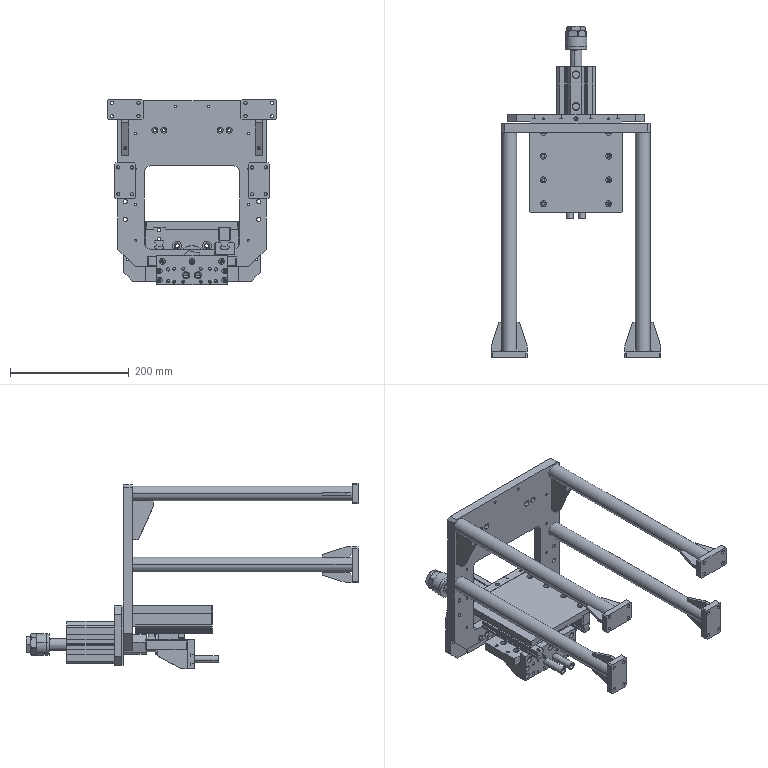Part | SolidWorks | features ReferencePattern 5, CompositeCurve 2, MirrorCompFeat 1 | 36 solids | 1817 faces | box 285 x 559 x 312.685 mm | volume 2790889 mm3 | plane 835 | cylinder 690 | cone 175 | spline 113 | sphere 4 | commonest cylinder face diameters 5.5 x102 4.5 x60 10 x56 8 x48 4.2 x42 0.8 x39